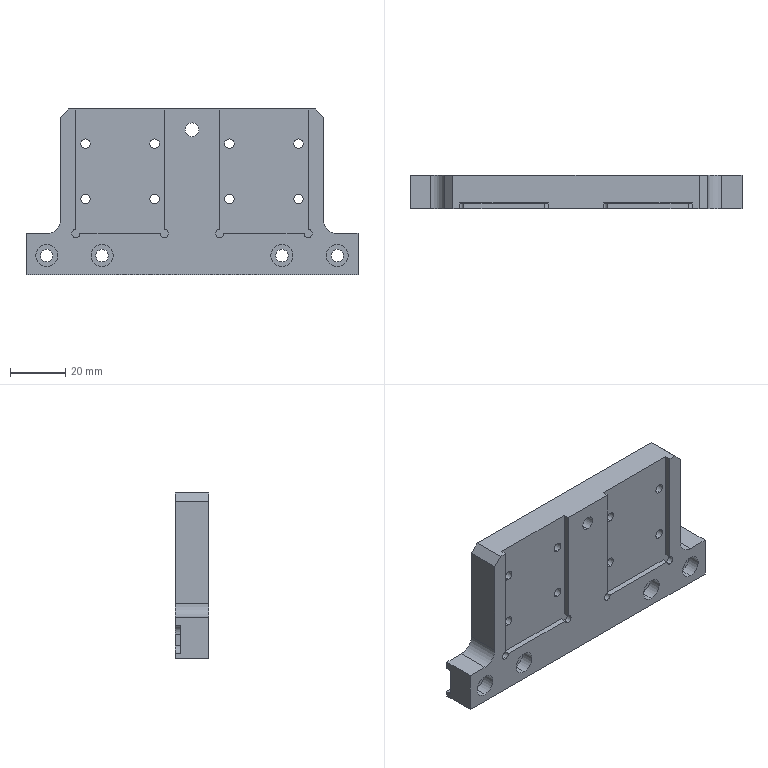Part | STEP file | PN_0017 | 1 solid | 104 faces | box 120 x 12 x 60 mm | volume 62781 mm3 | cylinder 64 | plane 40 | commonest cylinder face diameters 6 x20 3.4 x16 3 x8 4.5 x8 8 x8 5 x2